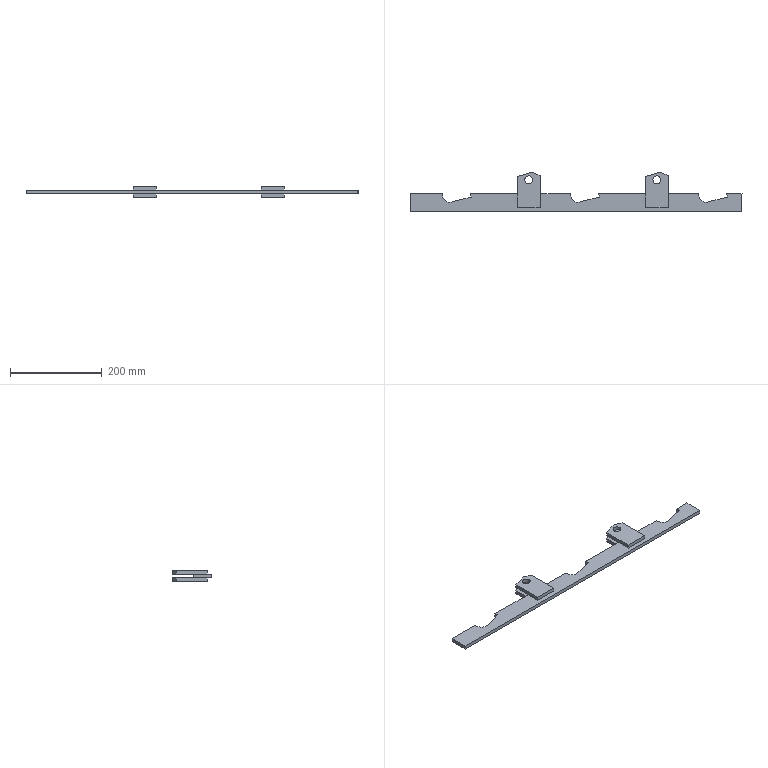Part | STEP file | Connecting plate assembly 1_Default<As machined> | 5 solids | 57 faces | box 725.342 x 86.845 x 24 mm | volume 319823 mm3 | plane 46 | cylinder 11 | commonest cylinder face diameters 17 x8 30 x3